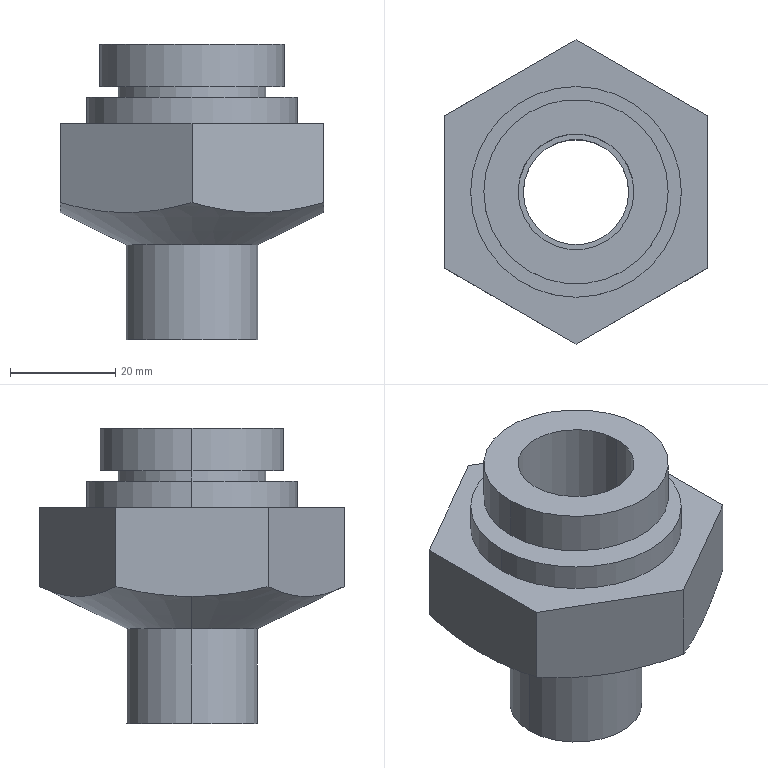Part | SolidWorks | features ICE 6, Extrusion 1, RevCut 1 | 1 solid | 26 faces | box 50 x 57.735 x 56 mm | volume 48059 mm3 | cylinder 12 | plane 12 | cone 2 | commonest cylinder face diameters 20 x2 22 x2 25 x2 28 x2 35 x2 40 x2
STEP:
#1=CARTESIAN_POINT('',(-10.,0.,-1.5));
#2=VERTEX_POINT('',#1);
#3=CARTESIAN_POINT('',(10.,0.,-1.5));
#4=VERTEX_POINT('',#3);
#5=CARTESIAN_POINT('',(0.,0.,-1.5));
#6=DIRECTION('',(0.,0.,1.));
#7=DIRECTION('',(1.,0.,0.));
#8=AXIS2_PLACEMENT_3D('',#5,#6,#7);
#9=CIRCLE('',#8,10.);
#10=EDGE_CURVE('',#2,#4,#9,.T.);
#11=ORIENTED_EDGE('',*,*,#10,.T.);
#12=CARTESIAN_POINT('',(10.,0.,-29.5));
#13=VERTEX_POINT('',#12);
#14=CARTESIAN_POINT('',(10.,0.,41.5));
#15=DIRECTION('',(0.,0.,-1.));
#16=VECTOR('',#15,1000.);
#17=LINE('',#14,#16);
#18=EDGE_CURVE('',#4,#13,#17,.T.);
#19=ORIENTED_EDGE('',*,*,#18,.T.);
#20=CARTESIAN_POINT('',(-10.,0.,-29.5));
#21=VERTEX_POINT('',#20);
#22=CARTESIAN_POINT('',(0.,0.,-29.5));
#23=DIRECTION('',(0.,0.,-1.));
#24=DIRECTION('',(-1.,0.,0.));
#25=AXIS2_PLACEMENT_3D('',#22,#23,#24);
#26=CIRCLE('',#25,10.);
#27=EDGE_CURVE('',#13,#21,#26,.T.);
#28=ORIENTED_EDGE('',*,*,#27,.T.);
#29=CARTESIAN_POINT('',(-10.,0.,41.5));
#30=DIRECTION('',(0.,0.,-1.));
#31=VECTOR('',#30,1000.);
#32=LINE('',#29,#31);
#33=EDGE_CURVE('',#2,#21,#32,.T.);
#34=ORIENTED_EDGE('',*,*,#33,.F.);
#35=EDGE_LOOP('',(#11,#19,#28,#34));
#36=FACE_OUTER_BOUND('',#35,.T.);
#37=CARTESIAN_POINT('',(0.,0.,41.5));
#38=DIRECTION('',(0.,0.,-1.));
#39=DIRECTION('',(-1.,0.,0.));
#40=AXIS2_PLACEMENT_3D('',#37,#38,#39);
#41=CYLINDRICAL_SURFACE('',#40,10.);
#42=ADVANCED_FACE('',(#36),#41,.F.);
#43=CARTESIAN_POINT('',(-11.,0.,-1.5));
#44=VERTEX_POINT('',#43);
#45=CARTESIAN_POINT('',(11.,0.,-1.5));
#46=VERTEX_POINT('',#45);
#47=CARTESIAN_POINT('',(0.,0.,-1.5));
#48=DIRECTION('',(0.,0.,1.));
#49=DIRECTION('',(1.,0.,0.));
#50=AXIS2_PLACEMENT_3D('',#47,#48,#49);
#51=CIRCLE('',#50,11.);
#52=EDGE_CURVE('',#44,#46,#51,.T.);
#53=ORIENTED_EDGE('',*,*,#52,.F.);
#54=CARTESIAN_POINT('',(-11.,0.,26.5));
#55=VERTEX_POINT('',#54);
#56=CARTESIAN_POINT('',(-11.,0.,-1.5));
#57=DIRECTION('',(0.,0.,1.));
#58=VECTOR('',#57,1000.);
#59=LINE('',#56,#58);
#60=EDGE_CURVE('',#44,#55,#59,.T.);
#61=ORIENTED_EDGE('',*,*,#60,.T.);
#62=CARTESIAN_POINT('',(11.,0.,26.5));
#63=VERTEX_POINT('',#62);
#64=CARTESIAN_POINT('',(0.,0.,26.5));
#65=DIRECTION('',(0.,0.,1.));
#66=DIRECTION('',(1.,0.,0.));
#67=AXIS2_PLACEMENT_3D('',#64,#65,#66);
#68=CIRCLE('',#67,11.);
#69=EDGE_CURVE('',#55,#63,#68,.T.);
#70=ORIENTED_EDGE('',*,*,#69,.T.);
#71=CARTESIAN_POINT('',(11.,0.,-1.5));
#72=DIRECTION('',(0.,0.,1.));
#73=VECTOR('',#72,1000.);
#74=LINE('',#71,#73);
#75=EDGE_CURVE('',#46,#63,#74,.T.);
#76=ORIENTED_EDGE('',*,*,#75,.F.);
#77=EDGE_LOOP('',(#53,#61,#70,#76));
#78=FACE_OUTER_BOUND('',#77,.T.);
#79=CARTESIAN_POINT('',(0.,0.,-1.5));
#80=DIRECTION('',(0.,0.,1.));
#81=DIRECTION('',(1.,0.,0.));
#82=AXIS2_PLACEMENT_3D('',#79,#80,#81);
#83=CYLINDRICAL_SURFACE('',#82,11.);
#84=ADVANCED_FACE('',(#78),#83,.F.);
#85=CARTESIAN_POINT('',(17.5,0.,26.5));
#86=VERTEX_POINT('',#85);
#87=CARTESIAN_POINT('',(-17.5,0.,26.5));
#88=VERTEX_POINT('',#87);
#89=CARTESIAN_POINT('',(0.,0.,26.5));
#90=DIRECTION('',(0.,0.,1.));
#91=DIRECTION('',(1.,0.,0.));
#92=AXIS2_PLACEMENT_3D('',#89,#90,#91);
#93=CIRCLE('',#92,17.5);
#94=EDGE_CURVE('',#86,#88,#93,.T.);
#95=ORIENTED_EDGE('',*,*,#94,.F.);
#96=CARTESIAN_POINT('',(17.5,0.,18.5));
#97=VERTEX_POINT('',#96);
#98=CARTESIAN_POINT('',(17.5,0.,26.5));
#99=DIRECTION('',(0.,0.,-1.));
#100=VECTOR('',#99,1000.);
#101=LINE('',#98,#100);
#102=EDGE_CURVE('',#86,#97,#101,.T.);
#103=ORIENTED_EDGE('',*,*,#102,.T.);
#104=CARTESIAN_POINT('',(-17.5,0.,18.5));
#105=VERTEX_POINT('',#104);
#106=CARTESIAN_POINT('',(0.,0.,18.5));
#107=DIRECTION('',(0.,0.,1.));
#108=DIRECTION('',(1.,0.,0.));
#109=AXIS2_PLACEMENT_3D('',#106,#107,#108);
#110=CIRCLE('',#109,17.5);
#111=EDGE_CURVE('',#97,#105,#110,.T.);
#112=ORIENTED_EDGE('',*,*,#111,.T.);
#113=CARTESIAN_POINT('',(-17.5,0.,26.5));
#114=DIRECTION('',(0.,0.,-1.));
#115=VECTOR('',#114,1000.);
#116=LINE('',#113,#115);
#117=EDGE_CURVE('',#88,#105,#116,.T.);
#118=ORIENTED_EDGE('',*,*,#117,.F.);
#119=EDGE_LOOP('',(#95,#103,#112,#118));
#120=FACE_OUTER_BOUND('',#119,.T.);
#121=CARTESIAN_POINT('',(0.,0.,26.5));
#122=DIRECTION('',(0.,0.,-1.));
#123=DIRECTION('',(-1.,0.,0.));
#124=AXIS2_PLACEMENT_3D('',#121,#122,#123);
#125=CYLINDRICAL_SURFACE('',#124,17.5);
#126=ADVANCED_FACE('',(#120),#125,.T.);
#127=CARTESIAN_POINT('',(14.,0.,18.5));
#128=VERTEX_POINT('',#127);
#129=CARTESIAN_POINT('',(-14.,0.,18.5));
#130=VERTEX_POINT('',#129);
#131=CARTESIAN_POINT('',(0.,0.,18.5));
#132=DIRECTION('',(0.,0.,1.));
#133=DIRECTION('',(1.,0.,0.));
#134=AXIS2_PLACEMENT_3D('',#131,#132,#133);
#135=CIRCLE('',#134,14.);
#136=EDGE_CURVE('',#128,#130,#135,.T.);
#137=ORIENTED_EDGE('',*,*,#136,.F.);
#138=CARTESIAN_POINT('',(14.,0.,16.5));
#139=VERTEX_POINT('',#138);
#140=CARTESIAN_POINT('',(14.,0.,18.5));
#141=DIRECTION('',(0.,0.,-1.));
#142=VECTOR('',#141,1000.);
#143=LINE('',#140,#142);
#144=EDGE_CURVE('',#128,#139,#143,.T.);
#145=ORIENTED_EDGE('',*,*,#144,.T.);
#146=CARTESIAN_POINT('',(-14.,0.,16.5));
#147=VERTEX_POINT('',#146);
#148=CARTESIAN_POINT('',(0.,0.,16.5));
#149=DIRECTION('',(0.,0.,1.));
#150=DIRECTION('',(1.,0.,0.));
#151=AXIS2_PLACEMENT_3D('',#148,#149,#150);
#152=CIRCLE('',#151,14.);
#153=EDGE_CURVE('',#139,#147,#152,.T.);
#154=ORIENTED_EDGE('',*,*,#153,.T.);
#155=CARTESIAN_POINT('',(-14.,0.,18.5));
#156=DIRECTION('',(0.,0.,-1.));
#157=VECTOR('',#156,1000.);
#158=LINE('',#155,#157);
#159=EDGE_CURVE('',#130,#147,#158,.T.);
#160=ORIENTED_EDGE('',*,*,#159,.F.);
#161=EDGE_LOOP('',(#137,#145,#154,#160));
#162=FACE_OUTER_BOUND('',#161,.T.);
#163=CARTESIAN_POINT('',(0.,0.,18.5));
#164=DIRECTION('',(0.,0.,-1.));
#165=DIRECTION('',(-1.,0.,0.));
#166=AXIS2_PLACEMENT_3D('',#163,#164,#165);
#167=CYLINDRICAL_SURFACE('',#166,14.);
#168=ADVANCED_FACE('',(#162),#167,.T.);
#169=CARTESIAN_POINT('',(20.,0.,16.5));
#170=VERTEX_POINT('',#169);
#171=CARTESIAN_POINT('',(-20.,0.,16.5));
#172=VERTEX_POINT('',#171);
#173=CARTESIAN_POINT('',(0.,0.,16.5));
#174=DIRECTION('',(0.,0.,1.));
#175=DIRECTION('',(1.,0.,0.));
#176=AXIS2_PLACEMENT_3D('',#173,#174,#175);
#177=CIRCLE('',#176,20.);
#178=EDGE_CURVE('',#170,#172,#177,.T.);
#179=ORIENTED_EDGE('',*,*,#178,.F.);
#180=CARTESIAN_POINT('',(20.,0.,11.5));
#181=VERTEX_POINT('',#180);
#182=CARTESIAN_POINT('',(20.,0.,16.5));
#183=DIRECTION('',(0.,0.,-1.));
#184=VECTOR('',#183,1000.);
#185=LINE('',#182,#184);
#186=EDGE_CURVE('',#170,#181,#185,.T.);
#187=ORIENTED_EDGE('',*,*,#186,.T.);
#188=CARTESIAN_POINT('',(-20.,0.,11.5));
#189=VERTEX_POINT('',#188);
#190=CARTESIAN_POINT('',(0.,0.,11.5));
#191=DIRECTION('',(0.,0.,1.));
#192=DIRECTION('',(1.,0.,0.));
#193=AXIS2_PLACEMENT_3D('',#190,#191,#192);
#194=CIRCLE('',#193,20.);
#195=EDGE_CURVE('',#181,#189,#194,.T.);
#196=ORIENTED_EDGE('',*,*,#195,.T.);
#197=CARTESIAN_POINT('',(-20.,0.,16.5));
#198=DIRECTION('',(0.,0.,-1.));
#199=VECTOR('',#198,1000.);
#200=LINE('',#197,#199);
#201=EDGE_CURVE('',#172,#189,#200,.T.);
#202=ORIENTED_EDGE('',*,*,#201,.F.);
#203=EDGE_LOOP('',(#179,#187,#196,#202));
#204=FACE_OUTER_BOUND('',#203,.T.);
#205=CARTESIAN_POINT('',(0.,0.,16.5));
#206=DIRECTION('',(0.,0.,-1.));
#207=DIRECTION('',(-1.,0.,0.));
#208=AXIS2_PLACEMENT_3D('',#205,#206,#207);
#209=CYLINDRICAL_SURFACE('',#208,20.);
#210=ADVANCED_FACE('',(#204),#209,.T.);
#211=CARTESIAN_POINT('',(-12.5,0.,-29.5));
#212=VERTEX_POINT('',#211);
#213=CARTESIAN_POINT('',(12.5,0.,-29.5));
#214=VERTEX_POINT('',#213);
#215=CARTESIAN_POINT('',(0.,0.,-29.5));
#216=DIRECTION('',(0.,0.,-1.));
#217=DIRECTION('',(-1.,0.,0.));
#218=AXIS2_PLACEMENT_3D('',#215,#216,#217);
#219=CIRCLE('',#218,12.5);
#220=EDGE_CURVE('',#212,#214,#219,.T.);
#221=ORIENTED_EDGE('',*,*,#220,.F.);
#222=CARTESIAN_POINT('',(-12.5,0.,-11.5));
#223=VERTEX_POINT('',#222);
#224=CARTESIAN_POINT('',(-12.5,0.,-29.5));
#225=DIRECTION('',(0.,0.,1.));
#226=VECTOR('',#225,1000.);
#227=LINE('',#224,#226);
#228=EDGE_CURVE('',#212,#223,#227,.T.);
#229=ORIENTED_EDGE('',*,*,#228,.T.);
#230=CARTESIAN_POINT('',(12.5,0.,-11.5));
#231=VERTEX_POINT('',#230);
#232=CARTESIAN_POINT('',(0.,0.,-11.5));
#233=DIRECTION('',(0.,0.,-1.));
#234=DIRECTION('',(-1.,0.,0.));
#235=AXIS2_PLACEMENT_3D('',#232,#233,#234);
#236=CIRCLE('',#235,12.5);
#237=EDGE_CURVE('',#223,#231,#236,.T.);
#238=ORIENTED_EDGE('',*,*,#237,.T.);
#239=CARTESIAN_POINT('',(12.5,0.,-29.5));
#240=DIRECTION('',(0.,0.,1.));
#241=VECTOR('',#240,1000.);
#242=LINE('',#239,#241);
#243=EDGE_CURVE('',#214,#231,#242,.T.);
#244=ORIENTED_EDGE('',*,*,#243,.F.);
#245=EDGE_LOOP('',(#221,#229,#238,#244));
#246=FACE_OUTER_BOUND('',#245,.T.);
#247=CARTESIAN_POINT('',(0.,0.,-29.5));
#248=DIRECTION('',(0.,0.,1.));
#249=DIRECTION('',(1.,0.,0.));
#250=AXIS2_PLACEMENT_3D('',#247,#248,#249);
#251=CYLINDRICAL_SURFACE('',#250,12.5);
#252=ADVANCED_FACE('',(#246),#251,.T.);
#253=ORIENTED_EDGE('',*,*,#237,.F.);
#254=CARTESIAN_POINT('',(-25.,0.,-5.39));
#255=VERTEX_POINT('',#254);
#256=CARTESIAN_POINT('',(-28.868,0.,-3.5));
#257=DIRECTION('',(-0.8984,0.,0.4391));
#258=VECTOR('',#257,1000.);
#259=LINE('',#256,#258);
#260=EDGE_CURVE('',#223,#255,#259,.T.);
#261=ORIENTED_EDGE('',*,*,#260,.T.);
#262=CARTESIAN_POINT('',(-25.,14.434,-3.5));
#263=VERTEX_POINT('',#262);
#264=CARTESIAN_POINT('',(-25.,0.,-5.39));
#265=CARTESIAN_POINT('',(-25.,2.418,-5.39));
#266=CARTESIAN_POINT('',(-25.,4.839,-5.216));
#267=CARTESIAN_POINT('',(-25.,7.87,-4.802));
#268=CARTESIAN_POINT('',(-25.,8.477,-4.71));
#269=CARTESIAN_POINT('',(-25.,9.683,-4.509));
#270=CARTESIAN_POINT('',(-25.,10.283,-4.4));
#271=CARTESIAN_POINT('',(-25.,12.075,-4.05));
#272=CARTESIAN_POINT('',(-25.,13.259,-3.787));
#273=CARTESIAN_POINT('',(-25.,14.434,-3.5));
#274=B_SPLINE_CURVE_WITH_KNOTS('',3,(#264,#265,#266,#267,#268,#269,#270,#271,#272,#273),.UNSPECIFIED.,.F.,.F.,(4,2,2,2,4),(0.03899,0.04628,0.0481,0.04993,0.05357),.UNSPECIFIED.);
#275=EDGE_CURVE('',#255,#263,#274,.T.);
#276=ORIENTED_EDGE('',*,*,#275,.T.);
#277=CARTESIAN_POINT('',(0.,28.868,-3.5));
#278=VERTEX_POINT('',#277);
#279=CARTESIAN_POINT('',(-25.,14.434,-3.5));
#280=CARTESIAN_POINT('',(-22.944,15.621,-4.08));
#281=CARTESIAN_POINT('',(-20.882,16.811,-4.555));
#282=CARTESIAN_POINT('',(-16.736,19.205,-5.209));
#283=CARTESIAN_POINT('',(-14.654,20.407,-5.387));
#284=CARTESIAN_POINT('',(-11.512,22.221,-5.392));
#285=CARTESIAN_POINT('',(-10.462,22.827,-5.35));
#286=CARTESIAN_POINT('',(-8.356,24.043,-5.182));
#287=CARTESIAN_POINT('',(-7.297,24.654,-5.055));
#288=CARTESIAN_POINT('',(-4.143,26.476,-4.561));
#289=CARTESIAN_POINT('',(-2.063,27.676,-4.082));
#290=CARTESIAN_POINT('',(0.,28.868,-3.5));
#291=B_SPLINE_CURVE_WITH_KNOTS('',3,(#279,#280,#281,#282,#283,#284,#285,#286,#287,#288,#289,#290),.UNSPECIFIED.,.F.,.F.,(4,2,2,2,2,4),(0.000000235,0.007234,0.01447,0.01809,0.0217,0.02894),.UNSPECIFIED.);
#292=EDGE_CURVE('',#263,#278,#291,.T.);
#293=ORIENTED_EDGE('',*,*,#292,.T.);
#294=CARTESIAN_POINT('',(25.,14.434,-3.5));
#295=VERTEX_POINT('',#294);
#296=CARTESIAN_POINT('',(0.,28.868,-3.5));
#297=CARTESIAN_POINT('',(2.056,27.681,-4.08));
#298=CARTESIAN_POINT('',(4.118,26.49,-4.555));
#299=CARTESIAN_POINT('',(8.264,24.097,-5.209));
#300=CARTESIAN_POINT('',(10.346,22.894,-5.387));
#301=CARTESIAN_POINT('',(13.488,21.08,-5.392));
#302=CARTESIAN_POINT('',(14.538,20.474,-5.35));
#303=CARTESIAN_POINT('',(16.644,19.258,-5.182));
#304=CARTESIAN_POINT('',(17.703,18.647,-5.055));
#305=CARTESIAN_POINT('',(20.857,16.826,-4.561));
#306=CARTESIAN_POINT('',(22.937,15.625,-4.082));
#307=CARTESIAN_POINT('',(25.,14.434,-3.5));
#308=B_SPLINE_CURVE_WITH_KNOTS('',3,(#296,#297,#298,#299,#300,#301,#302,#303,#304,#305,#306,#307),.UNSPECIFIED.,.F.,.F.,(4,2,2,2,2,4),(0.000000235,0.007234,0.01447,0.01809,0.0217,0.02894),.UNSPECIFIED.);
#309=EDGE_CURVE('',#278,#295,#308,.T.);
#310=ORIENTED_EDGE('',*,*,#309,.T.);
#311=CARTESIAN_POINT('',(25.,0.,-5.39));
#312=VERTEX_POINT('',#311);
#313=CARTESIAN_POINT('',(25.,14.434,-3.5));
#314=CARTESIAN_POINT('',(25.,13.259,-3.787));
#315=CARTESIAN_POINT('',(25.,12.075,-4.05));
#316=CARTESIAN_POINT('',(25.,10.283,-4.4));
#317=CARTESIAN_POINT('',(25.,9.683,-4.509));
#318=CARTESIAN_POINT('',(25.,8.477,-4.71));
#319=CARTESIAN_POINT('',(25.,7.87,-4.802));
#320=CARTESIAN_POINT('',(25.,4.839,-5.216));
#321=CARTESIAN_POINT('',(25.,2.418,-5.39));
#322=CARTESIAN_POINT('',(25.,0.,-5.39));
#323=B_SPLINE_CURVE_WITH_KNOTS('',3,(#313,#314,#315,#316,#317,#318,#319,#320,#321,#322),.UNSPECIFIED.,.F.,.F.,(4,2,2,2,4),(0.05217,0.05578,0.05758,0.05938,0.06659),.UNSPECIFIED.);
#324=EDGE_CURVE('',#295,#312,#323,.T.);
#325=ORIENTED_EDGE('',*,*,#324,.T.);
#326=CARTESIAN_POINT('',(28.868,0.,-3.5));
#327=DIRECTION('',(0.8984,0.,0.4391));
#328=VECTOR('',#327,1000.);
#329=LINE('',#326,#328);
#330=EDGE_CURVE('',#231,#312,#329,.T.);
#331=ORIENTED_EDGE('',*,*,#330,.F.);
#332=EDGE_LOOP('',(#253,#261,#276,#293,#310,#325,#331));
#333=FACE_OUTER_BOUND('',#332,.T.);
#334=CARTESIAN_POINT('',(0.,0.,-3.5));
#335=DIRECTION('',(0.,0.,1.));
#336=DIRECTION('',(1.,0.,0.));
#337=AXIS2_PLACEMENT_3D('',#334,#335,#336);
#338=CONICAL_SURFACE('',#337,28.868,1.116);
#339=ADVANCED_FACE('',(#333),#338,.T.);
#340=CARTESIAN_POINT('',(0.,0.,16.5));
#341=DIRECTION('',(0.,0.,1.));
#342=DIRECTION('',(1.,0.,0.));
#343=AXIS2_PLACEMENT_3D('',#340,#341,#342);
#344=CIRCLE('',#343,20.);
#345=EDGE_CURVE('',#172,#170,#344,.T.);
#346=ORIENTED_EDGE('',*,*,#345,.T.);
#347=ORIENTED_EDGE('',*,*,#178,.T.);
#348=EDGE_LOOP('',(#346,#347));
#349=FACE_OUTER_BOUND('',#348,.T.);
#350=CARTESIAN_POINT('',(0.,0.,16.5));
#351=DIRECTION('',(0.,0.,1.));
#352=DIRECTION('',(1.,0.,0.));
#353=AXIS2_PLACEMENT_3D('',#350,#351,#352);
#354=CIRCLE('',#353,14.);
#355=EDGE_CURVE('',#147,#139,#354,.T.);
#356=ORIENTED_EDGE('',*,*,#355,.F.);
#357=ORIENTED_EDGE('',*,*,#153,.F.);
#358=EDGE_LOOP('',(#356,#357));
#359=FACE_BOUND('',#358,.T.);
#360=CARTESIAN_POINT('',(0.,0.,16.5));
#361=DIRECTION('',(0.,0.,1.));
#362=DIRECTION('',(1.,0.,0.));
#363=AXIS2_PLACEMENT_3D('',#360,#361,#362);
#364=PLANE('',#363);
#365=ADVANCED_FACE('',(#349,#359),#364,.T.);
#366=CARTESIAN_POINT('',(25.,14.434,11.5));
#367=VERTEX_POINT('',#366);
#368=CARTESIAN_POINT('',(0.,28.868,11.5));
#369=VERTEX_POINT('',#368);
#370=CARTESIAN_POINT('',(25.,14.434,11.5));
#371=DIRECTION('',(-0.866,0.5,0.));
#372=VECTOR('',#371,1000.);
#373=LINE('',#370,#372);
#374=EDGE_CURVE('',#367,#369,#373,.T.);
#375=ORIENTED_EDGE('',*,*,#374,.T.);
#376=CARTESIAN_POINT('',(-25.,14.434,11.5));
#377=VERTEX_POINT('',#376);
#378=CARTESIAN_POINT('',(0.,28.868,11.5));
#379=DIRECTION('',(-0.866,-0.5,0.));
#380=VECTOR('',#379,1000.);
#381=LINE('',#378,#380);
#382=EDGE_CURVE('',#369,#377,#381,.T.);
#383=ORIENTED_EDGE('',*,*,#382,.T.);
#384=CARTESIAN_POINT('',(-25.,-14.434,11.5));
#385=VERTEX_POINT('',#384);
#386=CARTESIAN_POINT('',(-25.,14.434,11.5));
#387=DIRECTION('',(0.,-1.,0.));
#388=VECTOR('',#387,1000.);
#389=LINE('',#386,#388);
#390=EDGE_CURVE('',#377,#385,#389,.T.);
#391=ORIENTED_EDGE('',*,*,#390,.T.);
#392=CARTESIAN_POINT('',(0.,-28.868,11.5));
#393=VERTEX_POINT('',#392);
#394=CARTESIAN_POINT('',(-25.,-14.434,11.5));
#395=DIRECTION('',(0.866,-0.5,0.));
#396=VECTOR('',#395,1000.);
#397=LINE('',#394,#396);
#398=EDGE_CURVE('',#385,#393,#397,.T.);
#399=ORIENTED_EDGE('',*,*,#398,.T.);
#400=CARTESIAN_POINT('',(25.,-14.434,11.5));
#401=VERTEX_POINT('',#400);
#402=CARTESIAN_POINT('',(0.,-28.868,11.5));
#403=DIRECTION('',(0.866,0.5,0.));
#404=VECTOR('',#403,1000.);
#405=LINE('',#402,#404);
#406=EDGE_CURVE('',#393,#401,#405,.T.);
#407=ORIENTED_EDGE('',*,*,#406,.T.);
#408=CARTESIAN_POINT('',(25.,-14.434,11.5));
#409=DIRECTION('',(0.,1.,0.));
#410=VECTOR('',#409,1000.);
#411=LINE('',#408,#410);
#412=EDGE_CURVE('',#401,#367,#411,.T.);
#413=ORIENTED_EDGE('',*,*,#412,.T.);
#414=EDGE_LOOP('',(#375,#383,#391,#399,#407,#413));
#415=FACE_OUTER_BOUND('',#414,.T.);
#416=CARTESIAN_POINT('',(0.,0.,11.5));
#417=DIRECTION('',(0.,0.,1.));
#418=DIRECTION('',(1.,0.,0.));
#419=AXIS2_PLACEMENT_3D('',#416,#417,#418);
#420=CIRCLE('',#419,20.);
#421=EDGE_CURVE('',#189,#181,#420,.T.);
#422=ORIENTED_EDGE('',*,*,#421,.F.);
#423=ORIENTED_EDGE('',*,*,#195,.F.);
#424=EDGE_LOOP('',(#422,#423));
#425=FACE_BOUND('',#424,.T.);
#426=CARTESIAN_POINT('',(0.,0.,11.5));
#427=DIRECTION('',(0.,0.,1.));
#428=DIRECTION('',(1.,0.,0.));
#429=AXIS2_PLACEMENT_3D('',#426,#427,#428);
#430=PLANE('',#429);
#431=ADVANCED_FACE('',(#415,#425),#430,.T.);
#432=ORIENTED_EDGE('',*,*,#309,.F.);
#433=CARTESIAN_POINT('',(0.,28.868,11.5));
#434=DIRECTION('',(0.,0.,-1.));
#435=VECTOR('',#434,1000.);
#436=LINE('',#433,#435);
#437=EDGE_CURVE('',#369,#278,#436,.T.);
#438=ORIENTED_EDGE('',*,*,#437,.F.);
#439=ORIENTED_EDGE('',*,*,#374,.F.);
#440=CARTESIAN_POINT('',(25.,14.434,11.5));
#441=DIRECTION('',(0.,0.,-1.));
#442=VECTOR('',#441,1000.);
#443=LINE('',#440,#442);
#444=EDGE_CURVE('',#367,#295,#443,.T.);
#445=ORIENTED_EDGE('',*,*,#444,.T.);
#446=EDGE_LOOP('',(#432,#438,#439,#445));
#447=FACE_OUTER_BOUND('',#446,.T.);
#448=CARTESIAN_POINT('',(25.,14.434,11.5));
#449=DIRECTION('',(-0.5,-0.866,0.));
#450=DIRECTION('',(0.866,-0.5,0.));
#451=AXIS2_PLACEMENT_3D('',#448,#449,#450);
#452=PLANE('',#451);
#453=ADVANCED_FACE('',(#447),#452,.F.);
#454=ORIENTED_EDGE('',*,*,#292,.F.);
#455=CARTESIAN_POINT('',(-25.,14.434,11.5));
#456=DIRECTION('',(0.,0.,-1.));
#457=VECTOR('',#456,1000.);
#458=LINE('',#455,#457);
#459=EDGE_CURVE('',#377,#263,#458,.T.);
#460=ORIENTED_EDGE('',*,*,#459,.F.);
#461=ORIENTED_EDGE('',*,*,#382,.F.);
#462=ORIENTED_EDGE('',*,*,#437,.T.);
#463=EDGE_LOOP('',(#454,#460,#461,#462));
#464=FACE_OUTER_BOUND('',#463,.T.);
#465=CARTESIAN_POINT('',(0.,28.868,11.5));
#466=DIRECTION('',(0.5,-0.866,0.));
#467=DIRECTION('',(0.866,0.5,0.));
#468=AXIS2_PLACEMENT_3D('',#465,#466,#467);
#469=PLANE('',#468);
#470=ADVANCED_FACE('',(#464),#469,.F.);
#471=CARTESIAN_POINT('',(-25.,-14.434,-3.5));
#472=VERTEX_POINT('',#471);
#473=CARTESIAN_POINT('',(-25.,-14.434,-3.5));
#474=CARTESIAN_POINT('',(-25.,-13.25,-3.789));
#475=CARTESIAN_POINT('',(-25.,-12.059,-4.054));
#476=CARTESIAN_POINT('',(-25.,-9.657,-4.521));
#477=CARTESIAN_POINT('',(-25.,-8.449,-4.724));
#478=CARTESIAN_POINT('',(-25.,-4.832,-5.216));
#479=CARTESIAN_POINT('',(-25.,-2.418,-5.39));
#480=CARTESIAN_POINT('',(-25.,0.,-5.39));
#481=B_SPLINE_CURVE_WITH_KNOTS('',3,(#473,#474,#475,#476,#477,#478,#479,#480),.UNSPECIFIED.,.F.,.F.,(4,2,2,4),(0.02441,0.02806,0.0317,0.03899),.UNSPECIFIED.);
#482=EDGE_CURVE('',#472,#255,#481,.T.);
#483=ORIENTED_EDGE('',*,*,#482,.F.);
#484=CARTESIAN_POINT('',(-25.,-14.434,11.5));
#485=DIRECTION('',(0.,0.,-1.));
#486=VECTOR('',#485,1000.);
#487=LINE('',#484,#486);
#488=EDGE_CURVE('',#385,#472,#487,.T.);
#489=ORIENTED_EDGE('',*,*,#488,.F.);
#490=ORIENTED_EDGE('',*,*,#390,.F.);
#491=ORIENTED_EDGE('',*,*,#459,.T.);
#492=ORIENTED_EDGE('',*,*,#275,.F.);
#493=EDGE_LOOP('',(#483,#489,#490,#491,#492));
#494=FACE_OUTER_BOUND('',#493,.T.);
#495=CARTESIAN_POINT('',(-25.,14.434,11.5));
#496=DIRECTION('',(1.,0.,0.));
#497=DIRECTION('',(0.,1.,0.));
#498=AXIS2_PLACEMENT_3D('',#495,#496,#497);
#499=PLANE('',#498);
#500=ADVANCED_FACE('',(#494),#499,.F.);
#501=CARTESIAN_POINT('',(0.,-28.868,-3.5));
#502=VERTEX_POINT('',#501);
#503=CARTESIAN_POINT('',(0.,-28.868,-3.5));
#504=CARTESIAN_POINT('',(-2.056,-27.681,-4.08));
#505=CARTESIAN_POINT('',(-4.118,-26.49,-4.555));
#506=CARTESIAN_POINT('',(-8.264,-24.097,-5.209));
#507=CARTESIAN_POINT('',(-10.346,-22.894,-5.387));
#508=CARTESIAN_POINT('',(-13.488,-21.08,-5.392));
#509=CARTESIAN_POINT('',(-14.538,-20.474,-5.35));
#510=CARTESIAN_POINT('',(-16.644,-19.258,-5.182));
#511=CARTESIAN_POINT('',(-17.703,-18.647,-5.055));
#512=CARTESIAN_POINT('',(-20.857,-16.826,-4.561));
#513=CARTESIAN_POINT('',(-22.937,-15.625,-4.082));
#514=CARTESIAN_POINT('',(-25.,-14.434,-3.5));
#515=B_SPLINE_CURVE_WITH_KNOTS('',3,(#503,#504,#505,#506,#507,#508,#509,#510,#511,#512,#513,#514),.UNSPECIFIED.,.F.,.F.,(4,2,2,2,2,4),(0.000000235,0.007234,0.01447,0.01809,0.0217,0.02894),.UNSPECIFIED.);
#516=EDGE_CURVE('',#502,#472,#515,.T.);
#517=ORIENTED_EDGE('',*,*,#516,.F.);
#518=CARTESIAN_POINT('',(0.,-28.868,11.5));
#519=DIRECTION('',(0.,0.,-1.));
#520=VECTOR('',#519,1000.);
#521=LINE('',#518,#520);
#522=EDGE_CURVE('',#393,#502,#521,.T.);
#523=ORIENTED_EDGE('',*,*,#522,.F.);
#524=ORIENTED_EDGE('',*,*,#398,.F.);
#525=ORIENTED_EDGE('',*,*,#488,.T.);
#526=EDGE_LOOP('',(#517,#523,#524,#525));
#527=FACE_OUTER_BOUND('',#526,.T.);
#528=CARTESIAN_POINT('',(-25.,-14.434,11.5));
#529=DIRECTION('',(0.5,0.866,0.));
#530=DIRECTION('',(-0.866,0.5,0.));
#531=AXIS2_PLACEMENT_3D('',#528,#529,#530);
#532=PLANE('',#531);
#533=ADVANCED_FACE('',(#527),#532,.F.);
#534=CARTESIAN_POINT('',(25.,-14.434,-3.5));
#535=VERTEX_POINT('',#534);
#536=CARTESIAN_POINT('',(25.,-14.434,-3.5));
#537=CARTESIAN_POINT('',(22.944,-15.621,-4.08));
#538=CARTESIAN_POINT('',(20.882,-16.811,-4.555));
#539=CARTESIAN_POINT('',(16.736,-19.205,-5.209));
#540=CARTESIAN_POINT('',(14.654,-20.407,-5.387));
#541=CARTESIAN_POINT('',(11.512,-22.221,-5.392));
#542=CARTESIAN_POINT('',(10.462,-22.827,-5.35));
#543=CARTESIAN_POINT('',(8.356,-24.043,-5.182));
#544=CARTESIAN_POINT('',(7.297,-24.654,-5.055));
#545=CARTESIAN_POINT('',(4.143,-26.476,-4.561));
#546=CARTESIAN_POINT('',(2.063,-27.676,-4.082));
#547=CARTESIAN_POINT('',(0.,-28.868,-3.5));
#548=B_SPLINE_CURVE_WITH_KNOTS('',3,(#536,#537,#538,#539,#540,#541,#542,#543,#544,#545,#546,#547),.UNSPECIFIED.,.F.,.F.,(4,2,2,2,2,4),(0.000000235,0.007234,0.01447,0.01809,0.0217,0.02894),.UNSPECIFIED.);
#549=EDGE_CURVE('',#535,#502,#548,.T.);
#550=ORIENTED_EDGE('',*,*,#549,.F.);
#551=CARTESIAN_POINT('',(25.,-14.434,11.5));
#552=DIRECTION('',(0.,0.,-1.));
#553=VECTOR('',#552,1000.);
#554=LINE('',#551,#553);
#555=EDGE_CURVE('',#401,#535,#554,.T.);
#556=ORIENTED_EDGE('',*,*,#555,.F.);
#557=ORIENTED_EDGE('',*,*,#406,.F.);
#558=ORIENTED_EDGE('',*,*,#522,.T.);
#559=EDGE_LOOP('',(#550,#556,#557,#558));
#560=FACE_OUTER_BOUND('',#559,.T.);
#561=CARTESIAN_POINT('',(0.,-28.868,11.5));
#562=DIRECTION('',(-0.5,0.866,0.));
#563=DIRECTION('',(-0.866,-0.5,0.));
#564=AXIS2_PLACEMENT_3D('',#561,#562,#563);
#565=PLANE('',#564);
#566=ADVANCED_FACE('',(#560),#565,.F.);
#567=ORIENTED_EDGE('',*,*,#324,.F.);
#568=ORIENTED_EDGE('',*,*,#444,.F.);
#569=ORIENTED_EDGE('',*,*,#412,.F.);
#570=ORIENTED_EDGE('',*,*,#555,.T.);
#571=CARTESIAN_POINT('',(25.,0.,-5.39));
#572=CARTESIAN_POINT('',(25.,-2.418,-5.39));
#573=CARTESIAN_POINT('',(25.,-4.832,-5.216));
#574=CARTESIAN_POINT('',(25.,-8.449,-4.724));
#575=CARTESIAN_POINT('',(25.,-9.657,-4.521));
#576=CARTESIAN_POINT('',(25.,-12.059,-4.054));
#577=CARTESIAN_POINT('',(25.,-13.25,-3.789));
#578=CARTESIAN_POINT('',(25.,-14.434,-3.5));
#579=B_SPLINE_CURVE_WITH_KNOTS('',3,(#571,#572,#573,#574,#575,#576,#577,#578),.UNSPECIFIED.,.F.,.F.,(4,2,2,4),(0.06659,0.0738,0.0774,0.081),.UNSPECIFIED.);
#580=EDGE_CURVE('',#312,#535,#579,.T.);
#581=ORIENTED_EDGE('',*,*,#580,.F.);
#582=EDGE_LOOP('',(#567,#568,#569,#570,#581));
#583=FACE_OUTER_BOUND('',#582,.T.);
#584=CARTESIAN_POINT('',(25.,-14.434,11.5));
#585=DIRECTION('',(-1.,0.,0.));
#586=DIRECTION('',(0.,-1.,0.));
#587=AXIS2_PLACEMENT_3D('',#584,#585,#586);
#588=PLANE('',#587);
#589=ADVANCED_FACE('',(#583),#588,.F.);
#590=ORIENTED_EDGE('',*,*,#260,.F.);
#591=CARTESIAN_POINT('',(0.,0.,-11.5));
#592=DIRECTION('',(0.,0.,-1.));
#593=DIRECTION('',(-1.,0.,0.));
#594=AXIS2_PLACEMENT_3D('',#591,#592,#593);
#595=CIRCLE('',#594,12.5);
#596=EDGE_CURVE('',#231,#223,#595,.T.);
#597=ORIENTED_EDGE('',*,*,#596,.F.);
#598=ORIENTED_EDGE('',*,*,#330,.T.);
#599=ORIENTED_EDGE('',*,*,#580,.T.);
#600=ORIENTED_EDGE('',*,*,#549,.T.);
#601=ORIENTED_EDGE('',*,*,#516,.T.);
#602=ORIENTED_EDGE('',*,*,#482,.T.);
#603=EDGE_LOOP('',(#590,#597,#598,#599,#600,#601,#602));
#604=FACE_OUTER_BOUND('',#603,.T.);
#605=CARTESIAN_POINT('',(0.,0.,-3.5));
#606=DIRECTION('',(0.,0.,1.));
#607=DIRECTION('',(1.,0.,0.));
#608=AXIS2_PLACEMENT_3D('',#605,#606,#607);
#609=CONICAL_SURFACE('',#608,28.868,1.116);
#610=ADVANCED_FACE('',(#604),#609,.T.);
#611=ORIENTED_EDGE('',*,*,#228,.F.);
#612=CARTESIAN_POINT('',(0.,0.,-29.5));
#613=DIRECTION('',(0.,0.,-1.));
#614=DIRECTION('',(-1.,0.,0.));
#615=AXIS2_PLACEMENT_3D('',#612,#613,#614);
#616=CIRCLE('',#615,12.5);
#617=EDGE_CURVE('',#214,#212,#616,.T.);
#618=ORIENTED_EDGE('',*,*,#617,.F.);
#619=ORIENTED_EDGE('',*,*,#243,.T.);
#620=ORIENTED_EDGE('',*,*,#596,.T.);
#621=EDGE_LOOP('',(#611,#618,#619,#620));
#622=FACE_OUTER_BOUND('',#621,.T.);
#623=CARTESIAN_POINT('',(0.,0.,-29.5));
#624=DIRECTION('',(0.,0.,1.));
#625=DIRECTION('',(1.,0.,0.));
#626=AXIS2_PLACEMENT_3D('',#623,#624,#625);
#627=CYLINDRICAL_SURFACE('',#626,12.5);
#628=ADVANCED_FACE('',(#622),#627,.T.);
#629=CARTESIAN_POINT('',(0.,0.,-29.5));
#630=DIRECTION('',(0.,0.,-1.));
#631=DIRECTION('',(-1.,0.,0.));
#632=AXIS2_PLACEMENT_3D('',#629,#630,#631);
#633=CIRCLE('',#632,10.);
#634=EDGE_CURVE('',#21,#13,#633,.T.);
#635=ORIENTED_EDGE('',*,*,#634,.F.);
#636=ORIENTED_EDGE('',*,*,#27,.F.);
#637=EDGE_LOOP('',(#635,#636));
#638=FACE_BOUND('',#637,.T.);
#639=ORIENTED_EDGE('',*,*,#617,.T.);
#640=ORIENTED_EDGE('',*,*,#220,.T.);
#641=EDGE_LOOP('',(#639,#640));
#642=FACE_OUTER_BOUND('',#641,.T.);
#643=CARTESIAN_POINT('',(0.,0.,-29.5));
#644=DIRECTION('',(0.,0.,-1.));
#645=DIRECTION('',(-1.,0.,0.));
#646=AXIS2_PLACEMENT_3D('',#643,#644,#645);
#647=PLANE('',#646);
#648=ADVANCED_FACE('',(#638,#642),#647,.T.);
#649=ORIENTED_EDGE('',*,*,#186,.F.);
#650=ORIENTED_EDGE('',*,*,#345,.F.);
#651=ORIENTED_EDGE('',*,*,#201,.T.);
#652=ORIENTED_EDGE('',*,*,#421,.T.);
#653=EDGE_LOOP('',(#649,#650,#651,#652));
#654=FACE_OUTER_BOUND('',#653,.T.);
#655=CARTESIAN_POINT('',(0.,0.,16.5));
#656=DIRECTION('',(0.,0.,-1.));
#657=DIRECTION('',(-1.,0.,0.));
#658=AXIS2_PLACEMENT_3D('',#655,#656,#657);
#659=CYLINDRICAL_SURFACE('',#658,20.);
#660=ADVANCED_FACE('',(#654),#659,.T.);
#661=ORIENTED_EDGE('',*,*,#144,.F.);
#662=CARTESIAN_POINT('',(0.,0.,18.5));
#663=DIRECTION('',(0.,0.,1.));
#664=DIRECTION('',(1.,0.,0.));
#665=AXIS2_PLACEMENT_3D('',#662,#663,#664);
#666=CIRCLE('',#665,14.);
#667=EDGE_CURVE('',#130,#128,#666,.T.);
#668=ORIENTED_EDGE('',*,*,#667,.F.);
#669=ORIENTED_EDGE('',*,*,#159,.T.);
#670=ORIENTED_EDGE('',*,*,#355,.T.);
#671=EDGE_LOOP('',(#661,#668,#669,#670));
#672=FACE_OUTER_BOUND('',#671,.T.);
#673=CARTESIAN_POINT('',(0.,0.,18.5));
#674=DIRECTION('',(0.,0.,-1.));
#675=DIRECTION('',(-1.,0.,0.));
#676=AXIS2_PLACEMENT_3D('',#673,#674,#675);
#677=CYLINDRICAL_SURFACE('',#676,14.);
#678=ADVANCED_FACE('',(#672),#677,.T.);
#679=CARTESIAN_POINT('',(0.,0.,18.5));
#680=DIRECTION('',(0.,0.,1.));
#681=DIRECTION('',(1.,0.,0.));
#682=AXIS2_PLACEMENT_3D('',#679,#680,#681);
#683=CIRCLE('',#682,17.5);
#684=EDGE_CURVE('',#105,#97,#683,.T.);
#685=ORIENTED_EDGE('',*,*,#684,.F.);
#686=ORIENTED_EDGE('',*,*,#111,.F.);
#687=EDGE_LOOP('',(#685,#686));
#688=FACE_OUTER_BOUND('',#687,.T.);
#689=ORIENTED_EDGE('',*,*,#667,.T.);
#690=ORIENTED_EDGE('',*,*,#136,.T.);
#691=EDGE_LOOP('',(#689,#690));
#692=FACE_BOUND('',#691,.T.);
#693=CARTESIAN_POINT('',(0.,0.,18.5));
#694=DIRECTION('',(0.,0.,1.));
#695=DIRECTION('',(1.,0.,0.));
#696=AXIS2_PLACEMENT_3D('',#693,#694,#695);
#697=PLANE('',#696);
#698=ADVANCED_FACE('',(#688,#692),#697,.F.);
#699=ORIENTED_EDGE('',*,*,#102,.F.);
#700=CARTESIAN_POINT('',(0.,0.,26.5));
#701=DIRECTION('',(0.,0.,1.));
#702=DIRECTION('',(1.,0.,0.));
#703=AXIS2_PLACEMENT_3D('',#700,#701,#702);
#704=CIRCLE('',#703,17.5);
#705=EDGE_CURVE('',#88,#86,#704,.T.);
#706=ORIENTED_EDGE('',*,*,#705,.F.);
#707=ORIENTED_EDGE('',*,*,#117,.T.);
#708=ORIENTED_EDGE('',*,*,#684,.T.);
#709=EDGE_LOOP('',(#699,#706,#707,#708));
#710=FACE_OUTER_BOUND('',#709,.T.);
#711=CARTESIAN_POINT('',(0.,0.,26.5));
#712=DIRECTION('',(0.,0.,-1.));
#713=DIRECTION('',(-1.,0.,0.));
#714=AXIS2_PLACEMENT_3D('',#711,#712,#713);
#715=CYLINDRICAL_SURFACE('',#714,17.5);
#716=ADVANCED_FACE('',(#710),#715,.T.);
#717=CARTESIAN_POINT('',(0.,0.,26.5));
#718=DIRECTION('',(0.,0.,1.));
#719=DIRECTION('',(1.,0.,0.));
#720=AXIS2_PLACEMENT_3D('',#717,#718,#719);
#721=CIRCLE('',#720,11.);
#722=EDGE_CURVE('',#63,#55,#721,.T.);
#723=ORIENTED_EDGE('',*,*,#722,.F.);
#724=ORIENTED_EDGE('',*,*,#69,.F.);
#725=EDGE_LOOP('',(#723,#724));
#726=FACE_BOUND('',#725,.T.);
#727=ORIENTED_EDGE('',*,*,#705,.T.);
#728=ORIENTED_EDGE('',*,*,#94,.T.);
#729=EDGE_LOOP('',(#727,#728));
#730=FACE_OUTER_BOUND('',#729,.T.);
#731=CARTESIAN_POINT('',(0.,0.,26.5));
#732=DIRECTION('',(0.,0.,1.));
#733=DIRECTION('',(1.,0.,0.));
#734=AXIS2_PLACEMENT_3D('',#731,#732,#733);
#735=PLANE('',#734);
#736=ADVANCED_FACE('',(#726,#730),#735,.T.);
#737=ORIENTED_EDGE('',*,*,#60,.F.);
#738=CARTESIAN_POINT('',(0.,0.,-1.5));
#739=DIRECTION('',(0.,0.,1.));
#740=DIRECTION('',(1.,0.,0.));
#741=AXIS2_PLACEMENT_3D('',#738,#739,#740);
#742=CIRCLE('',#741,11.);
#743=EDGE_CURVE('',#46,#44,#742,.T.);
#744=ORIENTED_EDGE('',*,*,#743,.F.);
#745=ORIENTED_EDGE('',*,*,#75,.T.);
#746=ORIENTED_EDGE('',*,*,#722,.T.);
#747=EDGE_LOOP('',(#737,#744,#745,#746));
#748=FACE_OUTER_BOUND('',#747,.T.);
#749=CARTESIAN_POINT('',(0.,0.,-1.5));
#750=DIRECTION('',(0.,0.,1.));
#751=DIRECTION('',(1.,0.,0.));
#752=AXIS2_PLACEMENT_3D('',#749,#750,#751);
#753=CYLINDRICAL_SURFACE('',#752,11.);
#754=ADVANCED_FACE('',(#748),#753,.F.);
#755=ORIENTED_EDGE('',*,*,#10,.F.);
#756=CARTESIAN_POINT('',(0.,0.,-1.5));
#757=DIRECTION('',(0.,0.,1.));
#758=DIRECTION('',(1.,0.,0.));
#759=AXIS2_PLACEMENT_3D('',#756,#757,#758);
#760=CIRCLE('',#759,10.);
#761=EDGE_CURVE('',#4,#2,#760,.T.);
#762=ORIENTED_EDGE('',*,*,#761,.F.);
#763=EDGE_LOOP('',(#755,#762));
#764=FACE_BOUND('',#763,.T.);
#765=ORIENTED_EDGE('',*,*,#743,.T.);
#766=ORIENTED_EDGE('',*,*,#52,.T.);
#767=EDGE_LOOP('',(#765,#766));
#768=FACE_OUTER_BOUND('',#767,.T.);
#769=CARTESIAN_POINT('',(0.,0.,-1.5));
#770=DIRECTION('',(0.,0.,1.));
#771=DIRECTION('',(1.,0.,0.));
#772=AXIS2_PLACEMENT_3D('',#769,#770,#771);
#773=PLANE('',#772);
#774=ADVANCED_FACE('',(#764,#768),#773,.T.);
#775=ORIENTED_EDGE('',*,*,#18,.F.);
#776=ORIENTED_EDGE('',*,*,#761,.T.);
#777=ORIENTED_EDGE('',*,*,#33,.T.);
#778=ORIENTED_EDGE('',*,*,#634,.T.);
#779=EDGE_LOOP('',(#775,#776,#777,#778));
#780=FACE_OUTER_BOUND('',#779,.T.);
#781=CARTESIAN_POINT('',(0.,0.,41.5));
#782=DIRECTION('',(0.,0.,-1.));
#783=DIRECTION('',(-1.,0.,0.));
#784=AXIS2_PLACEMENT_3D('',#781,#782,#783);
#785=CYLINDRICAL_SURFACE('',#784,10.);
#786=ADVANCED_FACE('',(#780),#785,.F.);
#787=CLOSED_SHELL('',(#42,#84,#126,#168,#210,#252,#339,#365,#431,#453,#470,#500,#533,#566,#589,#610,#628,#648,#660,#678,#698,#716,#736,#754,#774,#786));
#788=MANIFOLD_SOLID_BREP('',#787);
#789=CARTESIAN_POINT('',(0.,0.,0.));
#790=DIRECTION('',(0.,0.,1.));
#791=DIRECTION('',(1.,0.,0.));
#792=AXIS2_PLACEMENT_3D('',#789,#790,#791);
#793=(LENGTH_UNIT()NAMED_UNIT(*)SI_UNIT(.MILLI.,.METRE.));
#794=UNCERTAINTY_MEASURE_WITH_UNIT(LENGTH_MEASURE(0.00001),#793,'','');
#795=(NAMED_UNIT(*)PLANE_ANGLE_UNIT()SI_UNIT($,.RADIAN.));
#796=(NAMED_UNIT(*)SI_UNIT($,.STERADIAN.)SOLID_ANGLE_UNIT());
#797=(GEOMETRIC_REPRESENTATION_CONTEXT(3)GLOBAL_UNCERTAINTY_ASSIGNED_CONTEXT((#794))GLOBAL_UNIT_ASSIGNED_CONTEXT((#793,#795,#796))REPRESENTATION_CONTEXT('',''));
#798=ADVANCED_BREP_SHAPE_REPRESENTATION('',(#788,#792),#797);